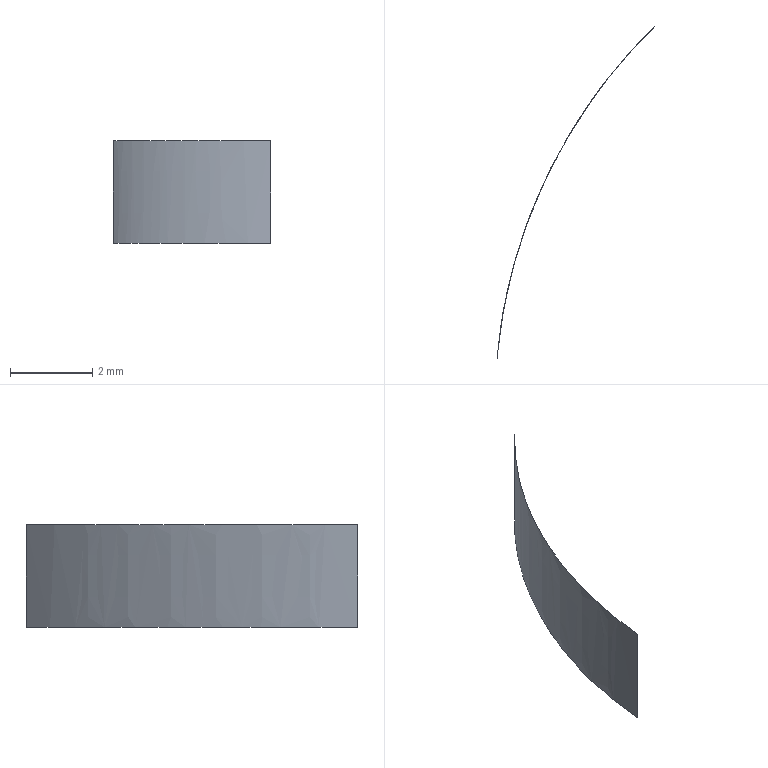Part | STEP file | lll_id382_x_t | 1 solid | 2 faces | box 3.844 x 8.077 x 2.5 mm | volume 0.01789 mm3 | other 1 | cylinder 1 | commonest cylinder face diameters 25.6 x1